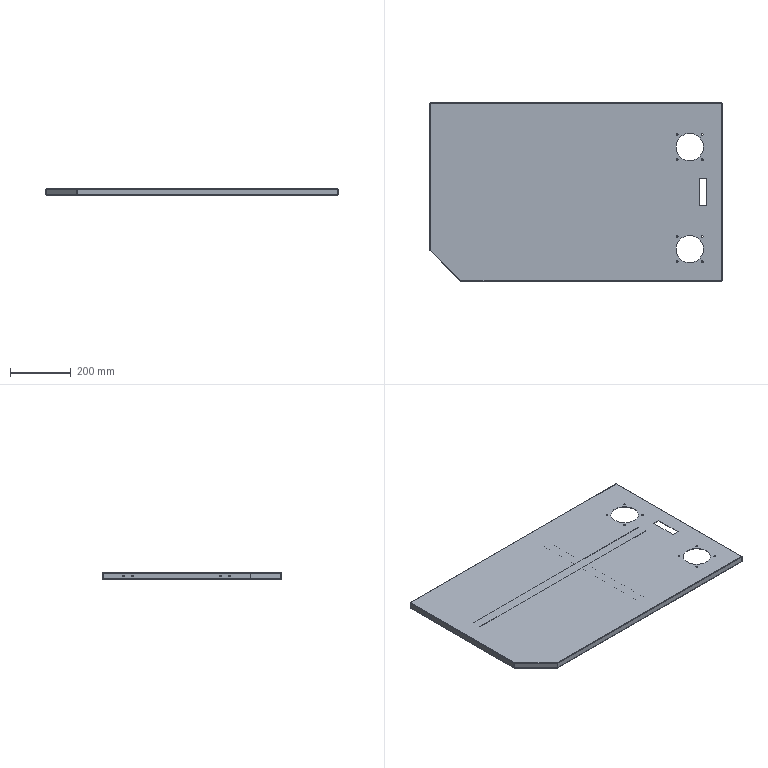Part | SolidWorks | features EdgeFlange 4, FlatPattern 4, SMBaseFlange 4, SheetMetal 4, HoleWzd 3, Cut 2, ICE 1 | 4 solids | 191 faces | box 959 x 587 x 21.5 mm | volume 1078977 mm3 | plane 101 | cylinder 70 | spline 20 | commonest cylinder face diameters 1.473 x16 4.473 x16 5.8 x16 3.3 x10 5 x8 90 x4